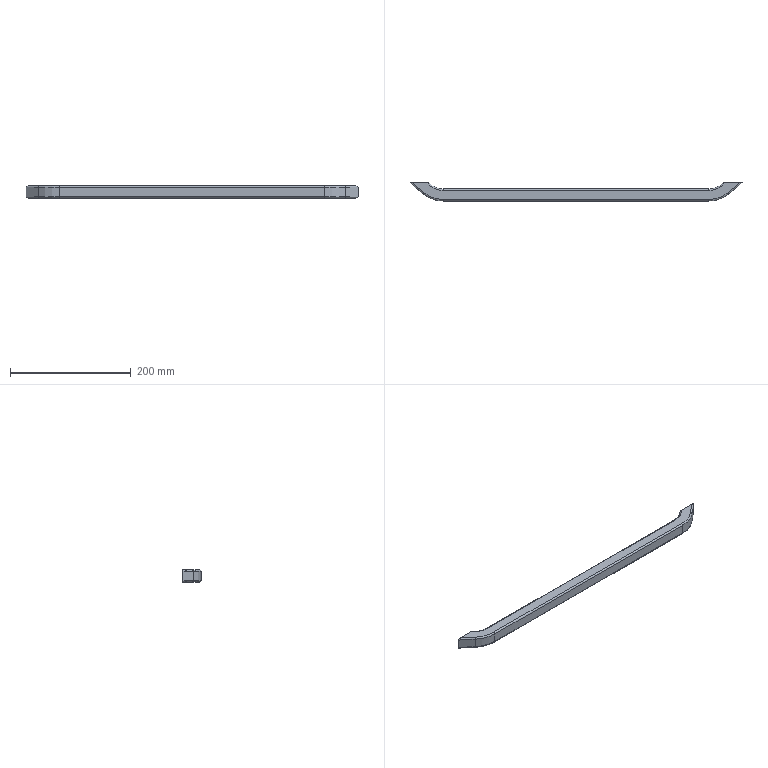Part | STEP file | 5090508 | 1 solid | 54 faces | box 550.086 x 30 x 20 mm | volume 56532 mm3 | cylinder 24 | torus 16 | plane 14 | commonest cylinder face diameters 2 x8 5 x8 66 x2 69 x2 103 x2 106 x2